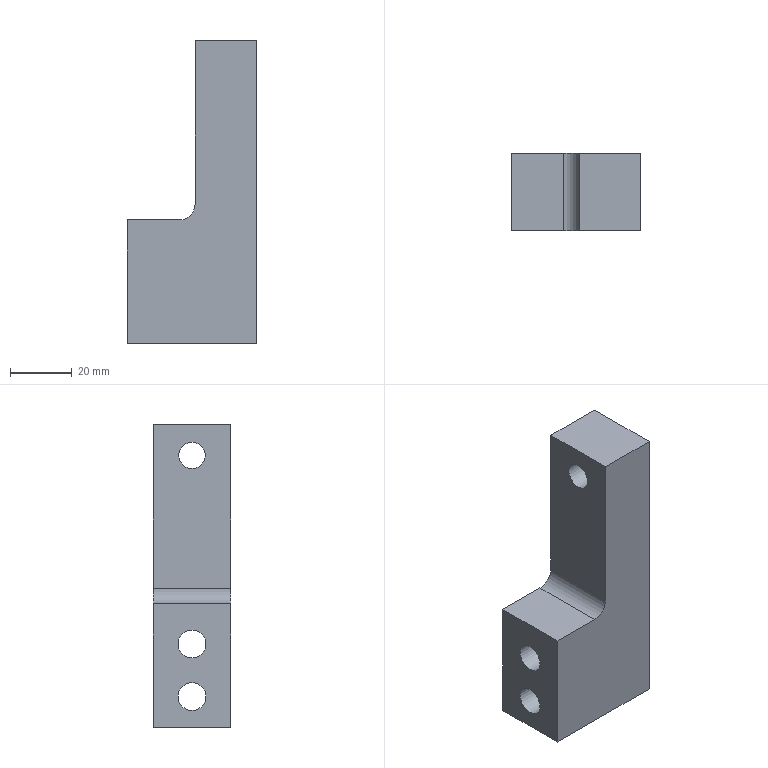Part | STEP file | 1 solid | 16 faces | box 42 x 25 x 98 mm | volume 60681 mm3 | plane 10 | cylinder 6 | commonest cylinder face diameters 9 x2 14 x2 8.5 x1 10 x1
STEP:
#1=CARTESIAN_POINT('',(382.,0.,5.25));
#2=VERTEX_POINT('',#1);
#3=CARTESIAN_POINT('',(382.,0.,1.));
#4=DIRECTION('',(-1.,0.,0.));
#5=DIRECTION('',(0.,0.,1.));
#6=AXIS2_PLACEMENT_3D('',#3,#4,#5);
#7=CIRCLE('',#6,4.25);
#8=EDGE_CURVE('',#2,#2,#7,.T.);
#9=ORIENTED_EDGE('',*,*,#8,.F.);
#10=EDGE_LOOP('',(#9));
#11=FACE_BOUND('',#10,.T.);
#12=CARTESIAN_POINT('',(382.,12.5,-42.));
#13=VERTEX_POINT('',#12);
#14=CARTESIAN_POINT('',(382.,12.5,11.));
#15=VERTEX_POINT('',#14);
#16=CARTESIAN_POINT('',(382.,12.5,-9.));
#17=DIRECTION('',(0.,0.,1.));
#18=VECTOR('',#17,1.);
#19=LINE('',#16,#18);
#20=EDGE_CURVE('',#13,#15,#19,.T.);
#21=ORIENTED_EDGE('',*,*,#20,.F.);
#22=CARTESIAN_POINT('',(382.,-12.5,-42.));
#23=VERTEX_POINT('',#22);
#24=CARTESIAN_POINT('',(382.,0.,-42.));
#25=DIRECTION('',(0.,-1.,0.));
#26=VECTOR('',#25,1.);
#27=LINE('',#24,#26);
#28=EDGE_CURVE('',#13,#23,#27,.T.);
#29=ORIENTED_EDGE('',*,*,#28,.T.);
#30=CARTESIAN_POINT('',(382.,-12.5,11.));
#31=VERTEX_POINT('',#30);
#32=CARTESIAN_POINT('',(382.,-12.5,11.));
#33=DIRECTION('',(0.,0.,1.));
#34=VECTOR('',#33,1.);
#35=LINE('',#32,#34);
#36=EDGE_CURVE('',#23,#31,#35,.T.);
#37=ORIENTED_EDGE('',*,*,#36,.T.);
#38=CARTESIAN_POINT('',(382.,12.5,11.));
#39=DIRECTION('',(0.,1.,0.));
#40=VECTOR('',#39,1.);
#41=LINE('',#38,#40);
#42=EDGE_CURVE('',#31,#15,#41,.T.);
#43=ORIENTED_EDGE('',*,*,#42,.T.);
#44=EDGE_LOOP('',(#21,#29,#37,#43));
#45=FACE_BOUND('',#44,.T.);
#46=CARTESIAN_POINT('',(382.,0.,26.));
#47=DIRECTION('',(-1.,0.,0.));
#48=DIRECTION('',(0.,0.,1.));
#49=AXIS2_PLACEMENT_3D('',#46,#47,#48);
#50=PLANE('',#49);
#51=ADVANCED_FACE('',(#11,#45),#50,.T.);
#52=CARTESIAN_POINT('',(360.,12.5,-87.));
#53=VERTEX_POINT('',#52);
#54=CARTESIAN_POINT('',(402.,12.5,-87.));
#55=VERTEX_POINT('',#54);
#56=CARTESIAN_POINT('',(88.5,12.5,-87.));
#57=DIRECTION('',(1.,0.,0.));
#58=VECTOR('',#57,1.);
#59=LINE('',#56,#58);
#60=EDGE_CURVE('',#53,#55,#59,.T.);
#61=ORIENTED_EDGE('',*,*,#60,.F.);
#62=CARTESIAN_POINT('',(360.,12.5,-47.));
#63=VERTEX_POINT('',#62);
#64=CARTESIAN_POINT('',(360.,12.5,-32.));
#65=DIRECTION('',(0.,0.,1.));
#66=VECTOR('',#65,1.);
#67=LINE('',#64,#66);
#68=EDGE_CURVE('',#53,#63,#67,.T.);
#69=ORIENTED_EDGE('',*,*,#68,.T.);
#70=CARTESIAN_POINT('',(377.,12.5,-47.));
#71=VERTEX_POINT('',#70);
#72=CARTESIAN_POINT('',(402.,12.5,-47.));
#73=DIRECTION('',(1.,0.,0.));
#74=VECTOR('',#73,1.);
#75=LINE('',#72,#74);
#76=EDGE_CURVE('',#63,#71,#75,.T.);
#77=ORIENTED_EDGE('',*,*,#76,.T.);
#78=CARTESIAN_POINT('',(377.,12.5,-42.));
#79=DIRECTION('',(0.,-1.,0.));
#80=DIRECTION('',(0.,0.,-1.));
#81=AXIS2_PLACEMENT_3D('',#78,#79,#80);
#82=CIRCLE('',#81,5.);
#83=EDGE_CURVE('',#71,#13,#82,.T.);
#84=ORIENTED_EDGE('',*,*,#83,.T.);
#85=ORIENTED_EDGE('',*,*,#20,.T.);
#86=CARTESIAN_POINT('',(402.,12.5,11.));
#87=VERTEX_POINT('',#86);
#88=CARTESIAN_POINT('',(402.,12.5,11.));
#89=DIRECTION('',(1.,0.,0.));
#90=VECTOR('',#89,1.);
#91=LINE('',#88,#90);
#92=EDGE_CURVE('',#15,#87,#91,.T.);
#93=ORIENTED_EDGE('',*,*,#92,.T.);
#94=CARTESIAN_POINT('',(402.,12.5,-9.));
#95=DIRECTION('',(0.,0.,1.));
#96=VECTOR('',#95,1.);
#97=LINE('',#94,#96);
#98=EDGE_CURVE('',#55,#87,#97,.T.);
#99=ORIENTED_EDGE('',*,*,#98,.F.);
#100=EDGE_LOOP('',(#61,#69,#77,#84,#85,#93,#99));
#101=FACE_OUTER_BOUND('',#100,.T.);
#102=CARTESIAN_POINT('',(402.,12.5,-9.));
#103=DIRECTION('',(0.,-1.,0.));
#104=DIRECTION('',(0.,0.,1.));
#105=AXIS2_PLACEMENT_3D('',#102,#103,#104);
#106=PLANE('',#105);
#107=ADVANCED_FACE('',(#101),#106,.F.);
#108=CARTESIAN_POINT('',(360.,-12.5,-87.));
#109=VERTEX_POINT('',#108);
#110=CARTESIAN_POINT('',(402.,-12.5,-87.));
#111=VERTEX_POINT('',#110);
#112=CARTESIAN_POINT('',(402.,-12.5,-87.));
#113=DIRECTION('',(1.,0.,0.));
#114=VECTOR('',#113,1.);
#115=LINE('',#112,#114);
#116=EDGE_CURVE('',#109,#111,#115,.T.);
#117=ORIENTED_EDGE('',*,*,#116,.F.);
#118=CARTESIAN_POINT('',(360.,0.,-87.));
#119=DIRECTION('',(0.,1.,0.));
#120=VECTOR('',#119,1.);
#121=LINE('',#118,#120);
#122=EDGE_CURVE('',#109,#53,#121,.T.);
#123=ORIENTED_EDGE('',*,*,#122,.T.);
#124=ORIENTED_EDGE('',*,*,#60,.T.);
#125=CARTESIAN_POINT('',(402.,15.,-87.));
#126=DIRECTION('',(0.,1.,0.));
#127=VECTOR('',#126,1.);
#128=LINE('',#125,#127);
#129=EDGE_CURVE('',#111,#55,#128,.T.);
#130=ORIENTED_EDGE('',*,*,#129,.F.);
#131=EDGE_LOOP('',(#117,#123,#124,#130));
#132=FACE_OUTER_BOUND('',#131,.T.);
#133=CARTESIAN_POINT('',(88.5,-1.,-87.));
#134=DIRECTION('',(0.,0.,1.));
#135=DIRECTION('',(1.,0.,0.));
#136=AXIS2_PLACEMENT_3D('',#133,#134,#135);
#137=PLANE('',#136);
#138=ADVANCED_FACE('',(#132),#137,.F.);
#139=ORIENTED_EDGE('',*,*,#36,.F.);
#140=CARTESIAN_POINT('',(377.,-12.5,-47.));
#141=VERTEX_POINT('',#140);
#142=CARTESIAN_POINT('',(377.,-12.5,-42.));
#143=DIRECTION('',(0.,1.,0.));
#144=DIRECTION('',(0.,0.,1.));
#145=AXIS2_PLACEMENT_3D('',#142,#143,#144);
#146=CIRCLE('',#145,5.);
#147=EDGE_CURVE('',#23,#141,#146,.T.);
#148=ORIENTED_EDGE('',*,*,#147,.T.);
#149=CARTESIAN_POINT('',(360.,-12.5,-47.));
#150=VERTEX_POINT('',#149);
#151=CARTESIAN_POINT('',(88.5,-12.5,-47.));
#152=DIRECTION('',(1.,0.,0.));
#153=VECTOR('',#152,1.);
#154=LINE('',#151,#153);
#155=EDGE_CURVE('',#150,#141,#154,.T.);
#156=ORIENTED_EDGE('',*,*,#155,.F.);
#157=CARTESIAN_POINT('',(360.,-12.5,-32.));
#158=DIRECTION('',(0.,0.,-1.));
#159=VECTOR('',#158,1.);
#160=LINE('',#157,#159);
#161=EDGE_CURVE('',#150,#109,#160,.T.);
#162=ORIENTED_EDGE('',*,*,#161,.T.);
#163=ORIENTED_EDGE('',*,*,#116,.T.);
#164=CARTESIAN_POINT('',(402.,-12.5,11.));
#165=VERTEX_POINT('',#164);
#166=CARTESIAN_POINT('',(402.,-12.5,11.));
#167=DIRECTION('',(0.,0.,-1.));
#168=VECTOR('',#167,1.);
#169=LINE('',#166,#168);
#170=EDGE_CURVE('',#165,#111,#169,.T.);
#171=ORIENTED_EDGE('',*,*,#170,.F.);
#172=CARTESIAN_POINT('',(402.,-12.5,11.));
#173=DIRECTION('',(1.,0.,0.));
#174=VECTOR('',#173,1.);
#175=LINE('',#172,#174);
#176=EDGE_CURVE('',#31,#165,#175,.T.);
#177=ORIENTED_EDGE('',*,*,#176,.F.);
#178=EDGE_LOOP('',(#139,#148,#156,#162,#163,#171,#177));
#179=FACE_OUTER_BOUND('',#178,.T.);
#180=CARTESIAN_POINT('',(402.,-12.5,11.));
#181=DIRECTION('',(0.,1.,0.));
#182=DIRECTION('',(0.,0.,-1.));
#183=AXIS2_PLACEMENT_3D('',#180,#181,#182);
#184=PLANE('',#183);
#185=ADVANCED_FACE('',(#179),#184,.F.);
#186=ORIENTED_EDGE('',*,*,#42,.F.);
#187=ORIENTED_EDGE('',*,*,#176,.T.);
#188=CARTESIAN_POINT('',(402.,12.5,11.));
#189=DIRECTION('',(0.,-1.,0.));
#190=VECTOR('',#189,1.);
#191=LINE('',#188,#190);
#192=EDGE_CURVE('',#87,#165,#191,.T.);
#193=ORIENTED_EDGE('',*,*,#192,.F.);
#194=ORIENTED_EDGE('',*,*,#92,.F.);
#195=EDGE_LOOP('',(#186,#187,#193,#194));
#196=FACE_OUTER_BOUND('',#195,.T.);
#197=CARTESIAN_POINT('',(402.,12.5,11.));
#198=DIRECTION('',(0.,0.,-1.));
#199=DIRECTION('',(0.,-1.,0.));
#200=AXIS2_PLACEMENT_3D('',#197,#198,#199);
#201=PLANE('',#200);
#202=ADVANCED_FACE('',(#196),#201,.F.);
#203=CARTESIAN_POINT('',(402.,0.,-53.));
#204=VERTEX_POINT('',#203);
#205=CARTESIAN_POINT('',(402.,0.,-60.));
#206=DIRECTION('',(-1.,0.,0.));
#207=DIRECTION('',(0.,0.,1.));
#208=AXIS2_PLACEMENT_3D('',#205,#206,#207);
#209=CIRCLE('',#208,7.);
#210=EDGE_CURVE('',#204,#204,#209,.T.);
#211=ORIENTED_EDGE('',*,*,#210,.T.);
#212=EDGE_LOOP('',(#211));
#213=FACE_BOUND('',#212,.T.);
#214=CARTESIAN_POINT('',(402.,0.,-70.));
#215=VERTEX_POINT('',#214);
#216=CARTESIAN_POINT('',(402.,0.,-77.));
#217=DIRECTION('',(-1.,0.,0.));
#218=DIRECTION('',(0.,0.,1.));
#219=AXIS2_PLACEMENT_3D('',#216,#217,#218);
#220=CIRCLE('',#219,7.);
#221=EDGE_CURVE('',#215,#215,#220,.T.);
#222=ORIENTED_EDGE('',*,*,#221,.T.);
#223=EDGE_LOOP('',(#222));
#224=FACE_BOUND('',#223,.T.);
#225=ORIENTED_EDGE('',*,*,#170,.T.);
#226=ORIENTED_EDGE('',*,*,#129,.T.);
#227=ORIENTED_EDGE('',*,*,#98,.T.);
#228=ORIENTED_EDGE('',*,*,#192,.T.);
#229=EDGE_LOOP('',(#225,#226,#227,#228));
#230=FACE_BOUND('',#229,.T.);
#231=CARTESIAN_POINT('',(402.,0.,5.25));
#232=VERTEX_POINT('',#231);
#233=CARTESIAN_POINT('',(402.,0.,1.));
#234=DIRECTION('',(-1.,0.,0.));
#235=DIRECTION('',(0.,0.,1.));
#236=AXIS2_PLACEMENT_3D('',#233,#234,#235);
#237=CIRCLE('',#236,4.25);
#238=EDGE_CURVE('',#232,#232,#237,.T.);
#239=ORIENTED_EDGE('',*,*,#238,.T.);
#240=EDGE_LOOP('',(#239));
#241=FACE_BOUND('',#240,.T.);
#242=CARTESIAN_POINT('',(402.,15.,-11.));
#243=DIRECTION('',(-1.,0.,0.));
#244=DIRECTION('',(0.,-1.,0.));
#245=AXIS2_PLACEMENT_3D('',#242,#243,#244);
#246=PLANE('',#245);
#247=ADVANCED_FACE('',(#213,#224,#230,#241),#246,.F.);
#248=CARTESIAN_POINT('',(360.,0.,-64.5));
#249=VERTEX_POINT('',#248);
#250=CARTESIAN_POINT('',(360.,0.,-60.));
#251=DIRECTION('',(1.,0.,0.));
#252=DIRECTION('',(0.,0.,-1.));
#253=AXIS2_PLACEMENT_3D('',#250,#251,#252);
#254=CIRCLE('',#253,4.5);
#255=EDGE_CURVE('',#249,#249,#254,.T.);
#256=ORIENTED_EDGE('',*,*,#255,.T.);
#257=EDGE_LOOP('',(#256));
#258=FACE_BOUND('',#257,.T.);
#259=CARTESIAN_POINT('',(360.,0.,-81.5));
#260=VERTEX_POINT('',#259);
#261=CARTESIAN_POINT('',(360.,0.,-77.));
#262=DIRECTION('',(1.,0.,0.));
#263=DIRECTION('',(0.,0.,-1.));
#264=AXIS2_PLACEMENT_3D('',#261,#262,#263);
#265=CIRCLE('',#264,4.5);
#266=EDGE_CURVE('',#260,#260,#265,.T.);
#267=ORIENTED_EDGE('',*,*,#266,.T.);
#268=EDGE_LOOP('',(#267));
#269=FACE_BOUND('',#268,.T.);
#270=ORIENTED_EDGE('',*,*,#161,.F.);
#271=CARTESIAN_POINT('',(360.,0.,-47.));
#272=DIRECTION('',(0.,-1.,0.));
#273=VECTOR('',#272,1.);
#274=LINE('',#271,#273);
#275=EDGE_CURVE('',#63,#150,#274,.T.);
#276=ORIENTED_EDGE('',*,*,#275,.F.);
#277=ORIENTED_EDGE('',*,*,#68,.F.);
#278=ORIENTED_EDGE('',*,*,#122,.F.);
#279=EDGE_LOOP('',(#270,#276,#277,#278));
#280=FACE_BOUND('',#279,.T.);
#281=CARTESIAN_POINT('',(360.,0.,-32.));
#282=DIRECTION('',(-1.,0.,0.));
#283=DIRECTION('',(0.,1.,0.));
#284=AXIS2_PLACEMENT_3D('',#281,#282,#283);
#285=PLANE('',#284);
#286=ADVANCED_FACE('',(#258,#269,#280),#285,.T.);
#287=ORIENTED_EDGE('',*,*,#155,.T.);
#288=CARTESIAN_POINT('',(377.,-1.,-47.));
#289=DIRECTION('',(0.,1.,0.));
#290=VECTOR('',#289,1.);
#291=LINE('',#288,#290);
#292=EDGE_CURVE('',#141,#71,#291,.T.);
#293=ORIENTED_EDGE('',*,*,#292,.T.);
#294=ORIENTED_EDGE('',*,*,#76,.F.);
#295=ORIENTED_EDGE('',*,*,#275,.T.);
#296=EDGE_LOOP('',(#287,#293,#294,#295));
#297=FACE_OUTER_BOUND('',#296,.T.);
#298=CARTESIAN_POINT('',(88.5,-1.,-47.));
#299=DIRECTION('',(0.,0.,1.));
#300=DIRECTION('',(1.,0.,0.));
#301=AXIS2_PLACEMENT_3D('',#298,#299,#300);
#302=PLANE('',#301);
#303=ADVANCED_FACE('',(#297),#302,.T.);
#304=ORIENTED_EDGE('',*,*,#83,.F.);
#305=ORIENTED_EDGE('',*,*,#292,.F.);
#306=ORIENTED_EDGE('',*,*,#147,.F.);
#307=ORIENTED_EDGE('',*,*,#28,.F.);
#308=EDGE_LOOP('',(#304,#305,#306,#307));
#309=FACE_OUTER_BOUND('',#308,.T.);
#310=CARTESIAN_POINT('',(377.,0.,-42.));
#311=DIRECTION('',(0.,1.,0.));
#312=DIRECTION('',(0.,0.,1.));
#313=AXIS2_PLACEMENT_3D('',#310,#311,#312);
#314=CYLINDRICAL_SURFACE('',#313,5.);
#315=ADVANCED_FACE('',(#309),#314,.F.);
#316=ORIENTED_EDGE('',*,*,#8,.T.);
#317=EDGE_LOOP('',(#316));
#318=FACE_BOUND('',#317,.T.);
#319=ORIENTED_EDGE('',*,*,#238,.F.);
#320=EDGE_LOOP('',(#319));
#321=FACE_BOUND('',#320,.T.);
#322=CARTESIAN_POINT('',(402.,0.,1.));
#323=DIRECTION('',(-1.,0.,0.));
#324=DIRECTION('',(0.,0.,-1.));
#325=AXIS2_PLACEMENT_3D('',#322,#323,#324);
#326=CYLINDRICAL_SURFACE('',#325,4.25);
#327=ADVANCED_FACE('',(#318,#321),#326,.F.);
#328=CARTESIAN_POINT('',(380.,0.,-72.5));
#329=VERTEX_POINT('',#328);
#330=CARTESIAN_POINT('',(380.,0.,-77.));
#331=DIRECTION('',(-1.,0.,0.));
#332=DIRECTION('',(0.,0.,1.));
#333=AXIS2_PLACEMENT_3D('',#330,#331,#332);
#334=CIRCLE('',#333,4.5);
#335=EDGE_CURVE('',#329,#329,#334,.T.);
#336=ORIENTED_EDGE('',*,*,#335,.F.);
#337=EDGE_LOOP('',(#336));
#338=FACE_BOUND('',#337,.T.);
#339=ORIENTED_EDGE('',*,*,#266,.F.);
#340=EDGE_LOOP('',(#339));
#341=FACE_BOUND('',#340,.T.);
#342=CARTESIAN_POINT('',(360.,0.,-77.));
#343=DIRECTION('',(1.,0.,0.));
#344=DIRECTION('',(0.,0.,-1.));
#345=AXIS2_PLACEMENT_3D('',#342,#343,#344);
#346=CYLINDRICAL_SURFACE('',#345,4.5);
#347=ADVANCED_FACE('',(#338,#341),#346,.F.);
#348=ORIENTED_EDGE('',*,*,#335,.T.);
#349=EDGE_LOOP('',(#348));
#350=FACE_BOUND('',#349,.T.);
#351=CARTESIAN_POINT('',(380.,0.,-84.));
#352=VERTEX_POINT('',#351);
#353=CARTESIAN_POINT('',(380.,0.,-77.));
#354=DIRECTION('',(-1.,0.,0.));
#355=DIRECTION('',(0.,0.,-1.));
#356=AXIS2_PLACEMENT_3D('',#353,#354,#355);
#357=CIRCLE('',#356,7.);
#358=EDGE_CURVE('',#352,#352,#357,.T.);
#359=ORIENTED_EDGE('',*,*,#358,.F.);
#360=EDGE_LOOP('',(#359));
#361=FACE_BOUND('',#360,.T.);
#362=CARTESIAN_POINT('',(380.,0.,-77.));
#363=DIRECTION('',(-1.,0.,0.));
#364=DIRECTION('',(0.,0.,1.));
#365=AXIS2_PLACEMENT_3D('',#362,#363,#364);
#366=PLANE('',#365);
#367=ADVANCED_FACE('',(#350,#361),#366,.F.);
#368=ORIENTED_EDGE('',*,*,#221,.F.);
#369=EDGE_LOOP('',(#368));
#370=FACE_BOUND('',#369,.T.);
#371=ORIENTED_EDGE('',*,*,#358,.T.);
#372=EDGE_LOOP('',(#371));
#373=FACE_BOUND('',#372,.T.);
#374=CARTESIAN_POINT('',(380.,0.,-77.));
#375=DIRECTION('',(1.,0.,0.));
#376=DIRECTION('',(0.,0.,-1.));
#377=AXIS2_PLACEMENT_3D('',#374,#375,#376);
#378=CYLINDRICAL_SURFACE('',#377,7.);
#379=ADVANCED_FACE('',(#370,#373),#378,.F.);
#380=CARTESIAN_POINT('',(380.,0.,-55.5));
#381=VERTEX_POINT('',#380);
#382=CARTESIAN_POINT('',(380.,0.,-60.));
#383=DIRECTION('',(-1.,0.,0.));
#384=DIRECTION('',(0.,0.,1.));
#385=AXIS2_PLACEMENT_3D('',#382,#383,#384);
#386=CIRCLE('',#385,4.5);
#387=EDGE_CURVE('',#381,#381,#386,.T.);
#388=ORIENTED_EDGE('',*,*,#387,.F.);
#389=EDGE_LOOP('',(#388));
#390=FACE_BOUND('',#389,.T.);
#391=ORIENTED_EDGE('',*,*,#255,.F.);
#392=EDGE_LOOP('',(#391));
#393=FACE_BOUND('',#392,.T.);
#394=CARTESIAN_POINT('',(360.,0.,-60.));
#395=DIRECTION('',(1.,0.,0.));
#396=DIRECTION('',(0.,0.,-1.));
#397=AXIS2_PLACEMENT_3D('',#394,#395,#396);
#398=CYLINDRICAL_SURFACE('',#397,4.5);
#399=ADVANCED_FACE('',(#390,#393),#398,.F.);
#400=ORIENTED_EDGE('',*,*,#387,.T.);
#401=EDGE_LOOP('',(#400));
#402=FACE_BOUND('',#401,.T.);
#403=CARTESIAN_POINT('',(380.,0.,-67.));
#404=VERTEX_POINT('',#403);
#405=CARTESIAN_POINT('',(380.,0.,-60.));
#406=DIRECTION('',(-1.,0.,0.));
#407=DIRECTION('',(0.,0.,-1.));
#408=AXIS2_PLACEMENT_3D('',#405,#406,#407);
#409=CIRCLE('',#408,7.);
#410=EDGE_CURVE('',#404,#404,#409,.T.);
#411=ORIENTED_EDGE('',*,*,#410,.F.);
#412=EDGE_LOOP('',(#411));
#413=FACE_BOUND('',#412,.T.);
#414=CARTESIAN_POINT('',(380.,0.,-60.));
#415=DIRECTION('',(-1.,0.,0.));
#416=DIRECTION('',(0.,0.,1.));
#417=AXIS2_PLACEMENT_3D('',#414,#415,#416);
#418=PLANE('',#417);
#419=ADVANCED_FACE('',(#402,#413),#418,.F.);
#420=ORIENTED_EDGE('',*,*,#210,.F.);
#421=EDGE_LOOP('',(#420));
#422=FACE_BOUND('',#421,.T.);
#423=ORIENTED_EDGE('',*,*,#410,.T.);
#424=EDGE_LOOP('',(#423));
#425=FACE_BOUND('',#424,.T.);
#426=CARTESIAN_POINT('',(380.,0.,-60.));
#427=DIRECTION('',(1.,0.,0.));
#428=DIRECTION('',(0.,0.,-1.));
#429=AXIS2_PLACEMENT_3D('',#426,#427,#428);
#430=CYLINDRICAL_SURFACE('',#429,7.);
#431=ADVANCED_FACE('',(#422,#425),#430,.F.);
#432=CLOSED_SHELL('',(#51,#107,#138,#185,#202,#247,#286,#303,#315,#327,#347,#367,#379,#399,#419,#431));
#433=MANIFOLD_SOLID_BREP('',#432);
#434=(LENGTH_UNIT()NAMED_UNIT(*)SI_UNIT(.MILLI.,.METRE.));
#435=UNCERTAINTY_MEASURE_WITH_UNIT(LENGTH_MEASURE(0.00002),#434,'','');
#436=(NAMED_UNIT(*)PLANE_ANGLE_UNIT()SI_UNIT($,.RADIAN.));
#437=PLANE_ANGLE_MEASURE_WITH_UNIT(PLANE_ANGLE_MEASURE(0.01745),#436);
#438=DIMENSIONAL_EXPONENTS(0.,0.,0.,0.,0.,0.,0.);
#439=(CONVERSION_BASED_UNIT('DEGREE',#437)NAMED_UNIT(#438)PLANE_ANGLE_UNIT());
#440=(NAMED_UNIT(*)SI_UNIT($,.STERADIAN.)SOLID_ANGLE_UNIT());
#441=(GEOMETRIC_REPRESENTATION_CONTEXT(3)GLOBAL_UNCERTAINTY_ASSIGNED_CONTEXT((#435))GLOBAL_UNIT_ASSIGNED_CONTEXT((#434,#439,#440))REPRESENTATION_CONTEXT('',''));
#442=ADVANCED_BREP_SHAPE_REPRESENTATION('',(#433),#441);